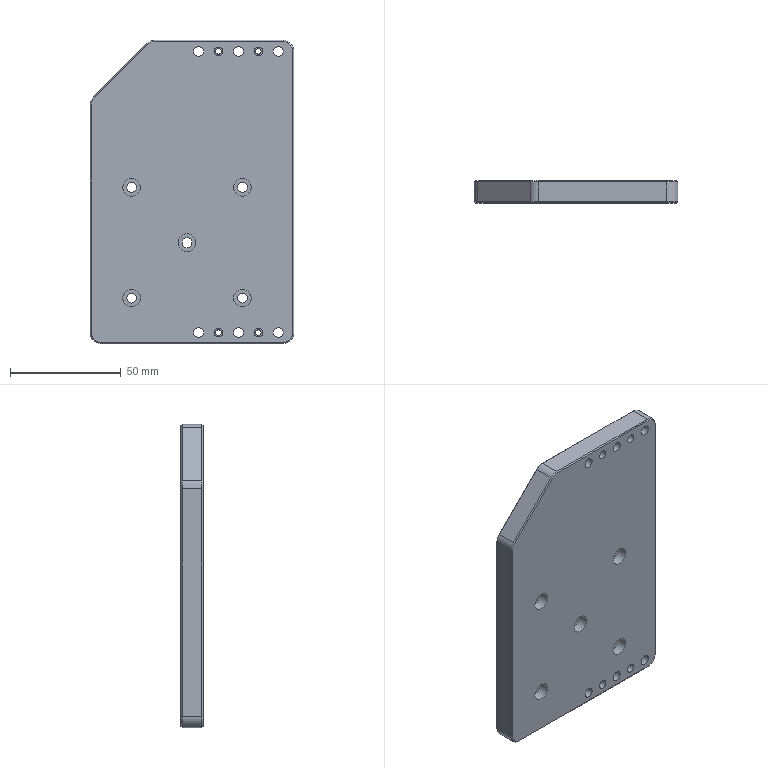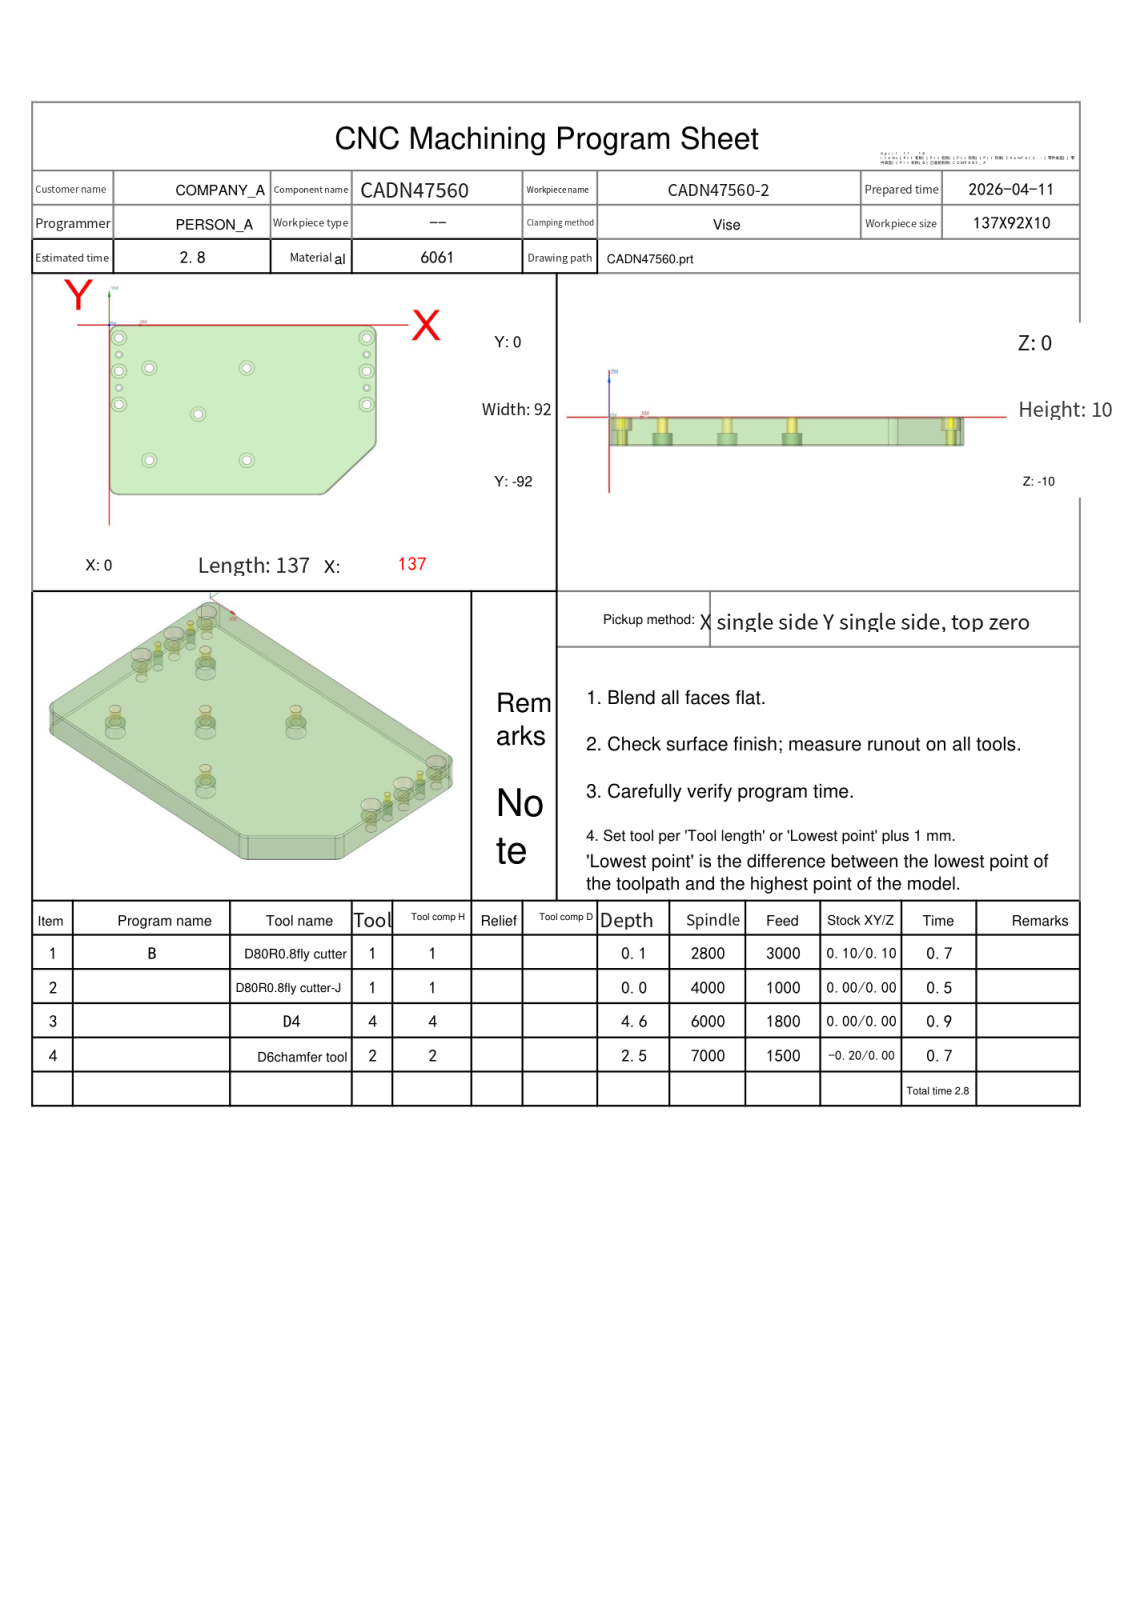NC program | NX | posted by the shop | part box 92 x 10 x 137 mm
Whole program:
%
O0001
(Machine time: 3.53 MIN)
(===Total Tool:3===)
(T1=D80R0.8 fly cutter D=80.  R=0.8  D-  H01 Z=0.    )
(T4=D4      D=4.   R=0.   D-  H04 Z=-4.6  )
(T2=D6chamfer tool   D=6.   R=0.   D-  H02 Z=-2.45 )
G80 G90 G17 G49 G40
G91 G28 Z0
M01
N1 T01 M06
(D80R0.8 fly cutter  D=80. R=0.8 H=01 ce=0.10 di=0.10)
G00 G90 G54 X188.863 Y-68.097 M03 S2800
G43 H01 Z20.
M08
Z3.525
G01 Z1.525 F3000.
X176.8
X-32.897
G02 X-40.097 Y-60.897 I0.0 J7.2
G01 Y-39.263
G02 X-32.097 Y-31.263 I8. J0.0
G01 X177.097
X189.097
Z3.525
G00 X188.863 Y-68.097
Z3.05
G01 Z1.05
X176.8
X-32.897
G02 X-40.097 Y-60.897 I0.0 J7.2
G01 Y-39.263
G02 X-32.097 Y-31.263 I8. J0.0
G01 X177.097
X189.097
Z3.05
G00 X188.863 Y-68.097
Z2.575
G01 Z.575
X176.8
X-32.897
G02 X-40.097 Y-60.897 I0.0 J7.2
G01 Y-39.263
G02 X-32.097 Y-31.263 I8. J0.0
G01 X177.097
X189.097
Z2.575
G00 X188.863 Y-68.097
Z2.1
G01 Z.1
X176.8
X-32.897
G02 X-40.097 Y-60.897 I0.0 J7.2
G01 Y-39.263
G02 X-32.097 Y-31.263 I8. J0.0
G01 X177.097
X189.097
Z2.1
G00 Z20.
G91 G28 Z0.0
M05
M09
G91 G28 Z0.0
M01
N2 T01 M06
(D80R0.8 fly cutter-J  D=80. R=0.8 H=01 ce=0.00 di=0.00)
G00 G90 G54 X188.773 Y-67.999 M03 S4000
G43 H01 Z20.
M08
Z2.
G01 Z0.0 F1000.
X176.712
X-32.799
G02 X-39.999 Y-60.799 I0.0 J7.2
G01 Y-39.361
G02 X-31.999 Y-31.361 I8. J0.0
G01 X176.999
X188.999
Z2.
G00 Z20.
G91 G28 Z0.0
M05
M09
G91 G28 Z0.0
M01
N3 T04 M06
(D4  D=4. R=0. H=04 ce=0.07 di=0.00)
G00 G90 G54 X132. Y-43. M03 S6000
G43 H04 Z20.
M08
Z.3
G03 X132.965 Y-42.035 I0.0 J.965 F1800.
X132. Y-41.07 I-.965 J0.0
X132. Y-41.07 Z-.05 I0.0 J-1.93
X132. Y-41.07 Z-.4 I0.0 J-1.93
X132. Y-41.07 Z-.75 I0.0 J-1.93
X132. Y-41.07 Z-1.1 I0.0 J-1.93
X132. Y-41.07 Z-1.45 I0.0 J-1.93
X132. Y-41.07 Z-1.8 I0.0 J-1.93
X132. Y-41.07 Z-2.15 I0.0 J-1.93
X132. Y-41.07 Z-2.5 I0.0 J-1.93
X132. Y-41.07 Z-2.85 I0.0 J-1.93
X132. Y-41.07 Z-3.2 I0.0 J-1.93
X132. Y-41.07 Z-3.55 I0.0 J-1.93
X132. Y-41.07 Z-3.9 I0.0 J-1.93
X132. Y-41.07 Z-4.25 I0.0 J-1.93
X132. Y-41.07 Z-4.6 I0.0 J-1.93
X130.07 Y-43. I0.0 J-1.93
X132. Y-44.93 I1.93 J0.0
X133.93 Y-43. I0.0 J1.93
X132. Y-41.07 I-1.93 J0.0
X131.035 Y-42.035 I0.0 J-.965
X132. Y-43. I.965 J0.0
G00 Z20.
Y-25.
Z.3
G03 X132.965 Y-24.035 I0.0 J.965
X132. Y-23.07 I-.965 J0.0
X132. Y-23.07 Z-.05 I0.0 J-1.93
X132. Y-23.07 Z-.4 I0.0 J-1.93
X132. Y-23.07 Z-.75 I0.0 J-1.93
X132. Y-23.07 Z-1.1 I0.0 J-1.93
X132. Y-23.07 Z-1.45 I0.0 J-1.93
X132. Y-23.07 Z-1.8 I0.0 J-1.93
X132. Y-23.07 Z-2.15 I0.0 J-1.93
X132. Y-23.07 Z-2.5 I0.0 J-1.93
X132. Y-23.07 Z-2.85 I0.0 J-1.93
X132. Y-23.07 Z-3.2 I0.0 J-1.93
X132. Y-23.07 Z-3.55 I0.0 J-1.93
X132. Y-23.07 Z-3.9 I0.0 J-1.93
X132. Y-23.07 Z-4.25 I0.0 J-1.93
X132. Y-23.07 Z-4.6 I0.0 J-1.93
X130.07 Y-25. I0.0 J-1.93
X132. Y-26.93 I1.93 J0.0
X133.93 Y-25. I0.0 J1.93
X132. Y-23.07 I-1.93 J0.0
X131.035 Y-24.035 I0.0 J-.965
X132. Y-25. I.965 J0.0
G00 Z20.
Y-7.
Z.3
G03 X132.965 Y-6.035 I0.0 J.965
X132. Y-5.07 I-.965 J0.0
X132. Y-5.07 Z-.05 I0.0 J-1.93
X132. Y-5.07 Z-.4 I0.0 J-1.93
X132. Y-5.07 Z-.75 I0.0 J-1.93
X132. Y-5.07 Z-1.1 I0.0 J-1.93
X132. Y-5.07 Z-1.45 I0.0 J-1.93
X132. Y-5.07 Z-1.8 I0.0 J-1.93
X132. Y-5.07 Z-2.15 I0.0 J-1.93
X132. Y-5.07 Z-2.5 I0.0 J-1.93
X132. Y-5.07 Z-2.85 I0.0 J-1.93
X132. Y-5.07 Z-3.2 I0.0 J-1.93
X132. Y-5.07 Z-3.55 I0.0 J-1.93
X132. Y-5.07 Z-3.9 I0.0 J-1.93
X132. Y-5.07 Z-4.25 I0.0 J-1.93
X132. Y-5.07 Z-4.6 I0.0 J-1.93
X130.07 Y-7. I0.0 J-1.93
X132. Y-8.93 I1.93 J0.0
X133.93 Y-7. I0.0 J1.93
X132. Y-5.07 I-1.93 J0.0
X131.035 Y-6.035 I0.0 J-.965
X132. Y-7. I.965 J0.0
G00 Z20.
X5.
Z.3
G03 X5.965 Y-6.035 I0.0 J.965
X5. Y-5.07 I-.965 J0.0
X5. Y-5.07 Z-.05 I0.0 J-1.93
X5. Y-5.07 Z-.4 I0.0 J-1.93
X5. Y-5.07 Z-.75 I0.0 J-1.93
X5. Y-5.07 Z-1.1 I0.0 J-1.93
X5. Y-5.07 Z-1.45 I0.0 J-1.93
X5. Y-5.07 Z-1.8 I0.0 J-1.93
X5. Y-5.07 Z-2.15 I0.0 J-1.93
X5. Y-5.07 Z-2.5 I0.0 J-1.93
X5. Y-5.07 Z-2.85 I0.0 J-1.93
X5. Y-5.07 Z-3.2 I0.0 J-1.93
X5. Y-5.07 Z-3.55 I0.0 J-1.93
X5. Y-5.07 Z-3.9 I0.0 J-1.93
X5. Y-5.07 Z-4.25 I0.0 J-1.93
X5. Y-5.07 Z-4.6 I0.0 J-1.93
X3.07 Y-7. I0.0 J-1.93
X5. Y-8.93 I1.93 J0.0
X6.93 Y-7. I0.0 J1.93
X5. Y-5.07 I-1.93 J0.0
X4.035 Y-6.035 I0.0 J-.965
X5. Y-7. I.965 J0.0
G00 Z20.
Y-25.
Z.3
G03 X5.965 Y-24.035 I0.0 J.965
X5. Y-23.07 I-.965 J0.0
X5. Y-23.07 Z-.05 I0.0 J-1.93
X5. Y-23.07 Z-.4 I0.0 J-1.93
X5. Y-23.07 Z-.75 I0.0 J-1.93
X5. Y-23.07 Z-1.1 I0.0 J-1.93
X5. Y-23.07 Z-1.45 I0.0 J-1.93
X5. Y-23.07 Z-1.8 I0.0 J-1.93
X5. Y-23.07 Z-2.15 I0.0 J-1.93
X5. Y-23.07 Z-2.5 I0.0 J-1.93
X5. Y-23.07 Z-2.85 I0.0 J-1.93
X5. Y-23.07 Z-3.2 I0.0 J-1.93
X5. Y-23.07 Z-3.55 I0.0 J-1.93
X5. Y-23.07 Z-3.9 I0.0 J-1.93
X5. Y-23.07 Z-4.25 I0.0 J-1.93
X5. Y-23.07 Z-4.6 I0.0 J-1.93
X3.07 Y-25. I0.0 J-1.93
X5. Y-26.93 I1.93 J0.0
X6.93 Y-25. I0.0 J1.93
X5. Y-23.07 I-1.93 J0.0
X4.035 Y-24.035 I0.0 J-.965
X5. Y-25. I.965 J0.0
G00 Z20.
Y-43.
Z.3
G03 X5.965 Y-42.035 I0.0 J.965
X5. Y-41.07 I-.965 J0.0
X5. Y-41.07 Z-.05 I0.0 J-1.93
X5. Y-41.07 Z-.4 I0.0 J-1.93
X5. Y-41.07 Z-.75 I0.0 J-1.93
X5. Y-41.07 Z-1.1 I0.0 J-1.93
X5. Y-41.07 Z-1.45 I0.0 J-1.93
X5. Y-41.07 Z-1.8 I0.0 J-1.93
X5. Y-41.07 Z-2.15 I0.0 J-1.93
X5. Y-41.07 Z-2.5 I0.0 J-1.93
X5. Y-41.07 Z-2.85 I0.0 J-1.93
X5. Y-41.07 Z-3.2 I0.0 J-1.93
X5. Y-41.07 Z-3.55 I0.0 J-1.93
X5. Y-41.07 Z-3.9 I0.0 J-1.93
X5. Y-41.07 Z-4.25 I0.0 J-1.93
X5. Y-41.07 Z-4.6 I0.0 J-1.93
X3.07 Y-43. I0.0 J-1.93
X5. Y-44.93 I1.93 J0.0
X6.93 Y-43. I0.0 J1.93
X5. Y-41.07 I-1.93 J0.0
X4.035 Y-42.035 I0.0 J-.965
X5. Y-43. I.965 J0.0
G00 Z20.
G00 G90 X132. Y-43. M03 S6000
Z20.
Z-4.6
G01 X132.329 Y-41.404 F600.
X132.336 Y-41.336
G03 X132. Y-41. I-.336 J0.0
X130. Y-43. I0.0 J-2.
X132. Y-45. I2. J0.0
X134. Y-43. I0.0 J2.
X132. Y-41. I-2. J0.0
X131.505 Y-41.062 I0.0 J-2.
X131.252 Y-41.388 I.083 J-.325
G01 X131.286 Y-41.535
X132. Y-43.
G00 Z20.
Y-25.
Z-4.6
G01 X132.329 Y-23.404
X132.336 Y-23.336
G03 X132. Y-23. I-.336 J0.0
X130. Y-25. I0.0 J-2.
X132. Y-27. I2. J0.0
X134. Y-25. I0.0 J2.
X132. Y-23. I-2. J0.0
X131.505 Y-23.062 I0.0 J-2.
X131.252 Y-23.388 I.083 J-.325
G01 X131.286 Y-23.535
X132. Y-25.
G00 Z20.
Y-7.
Z-4.6
G01 X132.329 Y-5.404
X132.336 Y-5.336
G03 X132. Y-5. I-.336 J0.0
X130. Y-7. I0.0 J-2.
X132. Y-9. I2. J0.0
X134. Y-7. I0.0 J2.
X132. Y-5. I-2. J0.0
X131.505 Y-5.062 I0.0 J-2.
X131.252 Y-5.388 I.083 J-.325
G01 X131.286 Y-5.535
X132. Y-7.
G00 Z20.
X5.
Z-4.6
G01 X5.329 Y-5.404
X5.336 Y-5.336
G03 X5. Y-5. I-.336 J0.0
X3. Y-7. I0.0 J-2.
X5. Y-9. I2. J0.0
X7. Y-7. I0.0 J2.
X5. Y-5. I-2. J0.0
X4.505 Y-5.062 I0.0 J-2.
X4.252 Y-5.388 I.083 J-.325
G01 X4.286 Y-5.535
X5. Y-7.
G00 Z20.
Y-25.
Z-4.6
G01 X5.329 Y-23.404
X5.336 Y-23.336
G03 X5. Y-23. I-.336 J0.0
X3. Y-25. I0.0 J-2.
X5. Y-27. I2. J0.0
X7. Y-25. I0.0 J2.
X5. Y-23. I-2. J0.0
X4.505 Y-23.062 I0.0 J-2.
X4.252 Y-23.388 I.083 J-.325
G01 X4.286 Y-23.535
X5. Y-25.
G00 Z20.
Y-43.
Z-4.6
G01 X5.329 Y-41.404
X5.336 Y-41.336
G03 X5. Y-41. I-.336 J0.0
X3. Y-43. I0.0 J-2.
X5. Y-45. I2. J0.0
X7. Y-43. I0.0 J2.
X5. Y-41. I-2. J0.0
X4.505 Y-41.062 I0.0 J-2.
X4.252 Y-41.388 I.083 J-.325
G01 X4.286 Y-41.535
X5. Y-43.
G00 Z20.
G91 G28 Z0.0
M05
M09
G91 G28 Z0.0
M01
N4 T02 M06
(D6chamfer tool  D=6. R=0. H=02 ce=0.00 di=0.00)
G00 G90 G54 X132. Y-34. M03 S7000
G43 H02 Z20.
M08
G98 G81 X132. Y-34. Z-1.75 R3. F500.
Y-16.
X5.
Y-34.
G80
G00 Z20.
G00 G90 X20.599 Y-23.25 M03 S7000
Z20.
G98 G81 X20.599 Y-23.25 Z-2.45 R3. F500.
X45.599 Y-48.25
X70.599 Y-23.25
Y-73.25
X20.599
G80
G00 Z20.
G00 G90 X132.507 Y-8.087 M03 S7000
Z20.
Z-1.5
G01 Z-2. F600.
X132.7 Y-8.5
G03 X134.2 Y-7. I0.0 J1.5
X132. Y-4.8 I-2.2 J0.0
X129.8 Y-7. I0.0 J-2.2
X132. Y-9.2 I2.2 J0.0
X134.2 Y-7. I0.0 J2.2
X132.7 Y-5.5 I-1.5 J0.0
G01 X132.507 Y-5.913
Z-1.5
G00 Z20.
Y-26.087
Z-1.5
G01 Z-2.
X132.7 Y-26.5
G03 X134.2 Y-25. I0.0 J1.5
X132. Y-22.8 I-2.2 J0.0
X129.8 Y-25. I0.0 J-2.2
X132. Y-27.2 I2.2 J0.0
X134.2 Y-25. I0.0 J2.2
X132.7 Y-23.5 I-1.5 J0.0
G01 X132.507 Y-23.913
Z-1.5
G00 Z20.
Y-44.087
Z-1.5
G01 Z-2.
X132.7 Y-44.5
G03 X134.2 Y-43. I0.0 J1.5
X132. Y-40.8 I-2.2 J0.0
X129.8 Y-43. I0.0 J-2.2
X132. Y-45.2 I2.2 J0.0
X134.2 Y-43. I0.0 J2.2
X132.7 Y-41.5 I-1.5 J0.0
G01 X132.507 Y-41.913
Z-1.5
G00 Z20.
X5.507 Y-44.087
Z-1.5
G01 Z-2.
X5.7 Y-44.5
G03 X7.2 Y-43. I0.0 J1.5
X5. Y-40.8 I-2.2 J0.0
X2.8 Y-43. I0.0 J-2.2
X5. Y-45.2 I2.2 J0.0
X7.2 Y-43. I0.0 J2.2
X5.7 Y-41.5 I-1.5 J0.0
G01 X5.507 Y-41.913
Z-1.5
G00 Z20.
Y-26.087
Z-1.5
G01 Z-2.
X5.7 Y-26.5
G03 X7.2 Y-25. I0.0 J1.5
X5. Y-22.8 I-2.2 J0.0
X2.8 Y-25. I0.0 J-2.2
X5. Y-27.2 I2.2 J0.0
X7.2 Y-25. I0.0 J2.2
X5.7 Y-23.5 I-1.5 J0.0
G01 X5.507 Y-23.913
Z-1.5
G00 Z20.
Y-8.087
Z-1.5
G01 Z-2.
X5.7 Y-8.5
G03 X7.2 Y-7. I0.0 J1.5
X5. Y-4.8 I-2.2 J0.0
X2.8 Y-7. I0.0 J-2.2
X5. Y-9.2 I2.2 J0.0
X7.2 Y-7. I0.0 J2.2
X5.7 Y-5.5 I-1.5 J0.0
G01 X5.507 Y-5.913
Z-1.5
G00 Z20.
G00 G90 X2.672 Y1.495 M03 S6500
Z20.
Z.3
G01 Z-1.2 F1500.
G03 X3.832 Y.6 I1.161 J.305
X4.035 Y.618 I0.0 J1.2
G01 X4.062 Y.622
G02 X5. Y.7 I.938 J-5.622
G01 X132.
G02 X137.7 Y-5. I0.0 J-5.7
G01 Y-62.929
G02 X136.031 Y-66.959 I-5.7 J0.0
G01 X111.959 Y-91.031
G02 X107.929 Y-92.7 I-4.031 J4.031
G01 X5.
G02 X-.7 Y-87. I0.0 J5.7
G01 Y-5.
G02 X4.035 Y.618 I5.7 J0.0
G01 X4.062 Y.622
G02 X4.432 Y.672 I.938 J-5.622
G03 X5.512 Y1.866 I-.12 J1.194
G01 X5.511 Y1.9
Z.3
G00 Z20.
M05
M09
G91 G28 Z0.0
G91 G28 Y0.0
M30
%